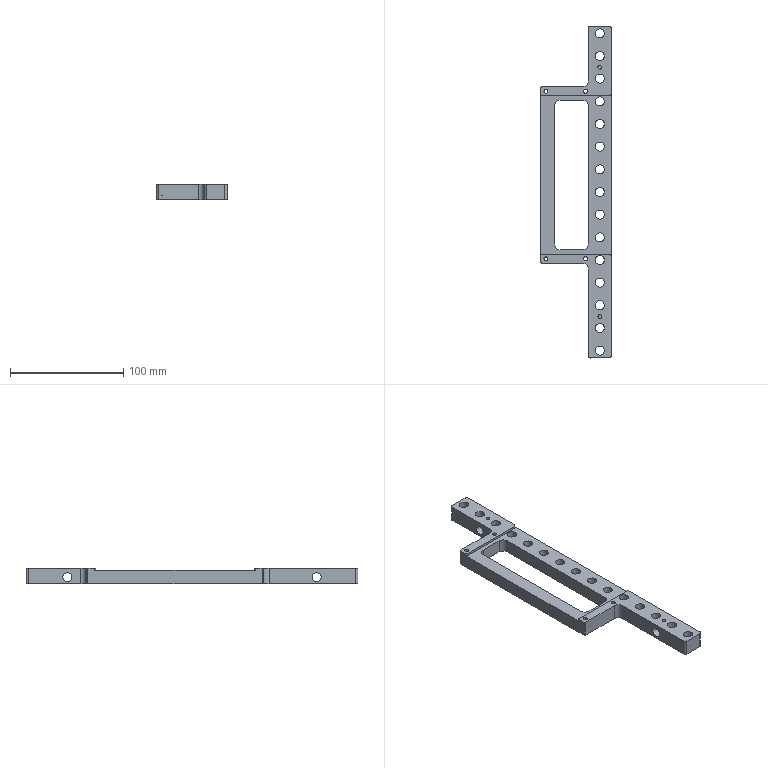CAM job | NX | 3-axis milling, drilling | part box 62 x 293 x 14 mm | stock box 65 x 298 x 20 mm
Tools:
number,name,description,diameter,corner_radius,flute_length,length,flutes
4,D4,平底铣刀-粗,4.0,0.0,25.0,75.0,2
9,D10,平底铣刀-粗,10.0,0.0,35.0,75.0,2
7,D6-J,平底铣刀-精,6.0,0.0,25.0,75.0,2
10,D10-J,平底铣刀-精,10.0,0.0,35.0,75.0,2
1,D80R0.8飞刀,圆鼻刀-粗,80.0,0.8,50.0,75.0,2
2,D6倒角刀,倒角刀,6.0,0.0,3.0,25.0,2
21,M4X0.7,丝锥,3.3,0.0,35.0,50.0,2
17,ZT3.5,钻头,3.5,0.0,35.0,50.0,2
18,ZT8.1,钻头,8.1,0.0,35.0,50.0,2
13,钻头3.3,Twist Drill 3.3 mm,3.3,0.0,35.0,35.008,2
Operations:
program,operation,operation_type,tool,method,geometry_group,spindle_rpm,surface_speed,feed_per_tooth,feed_cut,feed_plunge,cut_length_mm,path_length_mm,cut_time_min,machine_time_min
B,动态开粗D10_COPY_1,CavityMilling,D10,动态开粗-切深K-步距K,W-B,8000.0,251.32,0.25,4000.0,100.0,29481.421,29517.221,7.37,7.374
B,铣沉头_1,CylinderMilling,D4,METHOD,W-B,8000.0,100.531,0.075,1200.0,100.0,239.708,474.108,0.1998,0.2232
B,铣沉头_2,CylinderMilling,D4,METHOD,W-B,8000.0,100.531,0.075,1200.0,100.0,239.708,474.108,0.1998,0.2232
B,铣孔_1,CylinderMilling,D4,METHOD,W-B,8000.0,100.531,0.0375,600.0,100.0,18.52,260.519,0.0309,0.0551
B,铣孔_2,CylinderMilling,D4,METHOD,W-B,8000.0,100.531,0.0375,600.0,100.0,18.52,260.519,0.0309,0.0551
B,平面去毛刺6X45L_COPY,SurfaceContour,D6倒角刀,爬面_倒角-切深0-步距G,W-B,6500.0,122.519,0.1154,1500.0,100.0,1446.187,2516.183,0.9641,1.071
B,底壁铣飞面精光_COPY,VolumeBased25DMillingOperation,D10-J,侧刃精光-切深K-步距G,W-B,8000.0,251.32,0.0625,1000.0,100.0,2188.08,2224.08,2.188,2.192
A,顶面,FaceMilling,D80R0.8飞刀,侧刃精光-切深K-步距G,W-A,4000.0,1005.31,0.125,1000.0,100.0,387.0,423.0,0.387,0.3906
A,动态开粗D10_COPY,CavityMilling,D10,动态开粗-切深K-步距K,W-A,8000.0,251.327,0.2188,3500.0,100.0,30277.447,30741.248,8.651,8.697
A,打点-深0.8,Operation,D6倒角刀,NONE,W-A,8000.0,150.796,0.0312,500.0,90.0,37.8,574.107,0.0756,0.1292
A,通孔-3-4,Operation,ZT3.5,NONE,W-A,3000.0,32.987,0.0417,250.0,90.0,76.0,413.032,0.304,0.3377
A,通孔-8-10,Operation,ZT8.1,NONE,W-A,1800.0,45.804,0.0833,300.0,90.0,277.502,889.553,0.925,0.9862
A,盲锥孔-M4螺纹底孔,Operation,钻头3.3,NONE,W-A,3000.0,31.102,0.02,120.0,90.0,25.0,311.002,0.2083,0.2369
A,底精_1,VolumeBased25DMillingOperation,D6-J,METHOD,W-A,6000.0,113.0,0.2083,1200.0,100.0,2324.951,2608.559,1.938,1.966
A,仅选体,SurfaceContour,D6倒角刀,METHOD,W-A,8000.0,150.796,0.1875,3000.0,100.0,1188.244,1775.202,0.3961,0.4548
A,钻倒角_1,Operation,D6倒角刀,METHOD,W-A,8000.0,150.796,0.0312,500.0,0.0,10.4,283.82,0.0208,0.0481
A,钻倒角_2,Operation,D6倒角刀,METHOD,W-A,8000.0,150.796,0.0312,500.0,0.0,20.2,307.687,0.0404,0.0691
A,铣倒角_1,PlanarMilling,D6倒角刀,METHOD,W-A,8000.0,150.796,0.05,800.0,100.0,391.312,1329.131,0.4891,0.5829
A,盲锥孔-攻牙M4,Operation,M4X0.7,METHOD,W-A,800.0,8.294,0.0004,0.7,90.0,18.0,297.002,25.714,25.742
A,底侧精_3,VolumeBased25DMillingOperation,D6-J,METHOD,W-A,6000.0,113.0,0.2083,1200.0,100.0,165.757,401.137,0.1381,0.1617
A,框精_1,VolumeBased25DMillingOperation,D6-J,METHOD,W-A,6000.0,113.0,0.0833,1000.0,100.0,301.878,368.878,0.3019,0.3086
A,外形半精_2,VolumeBased25DMillingOperation,D10-J,METHOD,W-A,8000.0,251.327,0.0625,1000.0,100.0,737.725,805.325,0.7377,0.7445